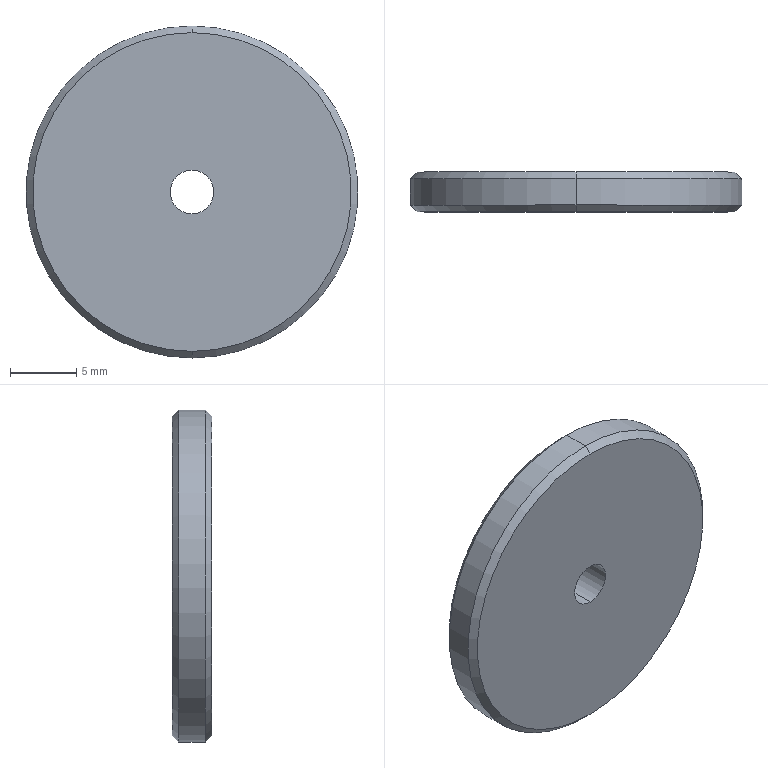Part | STEP file | ND25021-01-JDKM-13-BJ | 1 solid | 10 faces | box 25 x 3 x 25 mm | volume 1428 mm3 | cylinder 4 | cone 4 | plane 2 | commonest cylinder face diameters 3.3 x2 25 x2
STEP:
#1=CARTESIAN_POINT('',(0.,0.,0.));
#2=DIRECTION('',(0.,0.,1.));
#3=DIRECTION('',(1.,0.,0.));
#4=AXIS2_PLACEMENT_3D('',#1,#2,#3);
#5=CARTESIAN_POINT('',(0.,0.,1.65));
#6=VERTEX_POINT('',#5);
#7=CARTESIAN_POINT('',(0.,3.,1.65));
#8=VERTEX_POINT('',#7);
#9=CARTESIAN_POINT('',(0.,3.,1.65));
#10=DIRECTION('',(0.,1.,0.));
#11=VECTOR('',#10,1.);
#12=LINE('',#9,#11);
#13=CARTESIAN_POINT('',(0.,3.,0.));
#14=DIRECTION('',(0.,1.,0.));
#15=DIRECTION('',(0.,0.,1.));
#16=AXIS2_PLACEMENT_3D('',#13,#14,#15);
#17=CYLINDRICAL_SURFACE('',#16,1.65);
#18=CARTESIAN_POINT('',(6.283,0.));
#19=DIRECTION('',(0.,1.));
#20=VECTOR('',#19,1.);
#21=LINE('',#18,#20);
#22=(GEOMETRIC_REPRESENTATION_CONTEXT(2)PARAMETRIC_REPRESENTATION_CONTEXT()REPRESENTATION_CONTEXT('',''));
#23=DEFINITIONAL_REPRESENTATION('',(#21),#22);
#24=PCURVE('',#17,#23);
#25=CARTESIAN_POINT('',(0.,3.,0.));
#26=DIRECTION('',(0.,1.,0.));
#27=DIRECTION('',(0.,0.,1.));
#28=AXIS2_PLACEMENT_3D('',#25,#26,#27);
#29=CYLINDRICAL_SURFACE('',#28,1.65);
#30=CARTESIAN_POINT('',(0.,0.));
#31=DIRECTION('',(0.,1.));
#32=VECTOR('',#31,1.);
#33=LINE('',#30,#32);
#34=(GEOMETRIC_REPRESENTATION_CONTEXT(2)PARAMETRIC_REPRESENTATION_CONTEXT()REPRESENTATION_CONTEXT('',''));
#35=DEFINITIONAL_REPRESENTATION('',(#33),#34);
#36=PCURVE('',#29,#35);
#37=SURFACE_CURVE('',#12,(#24,#36),.PCURVE_S1.);
#38=EDGE_CURVE('',#6,#8,#37,.T.);
#39=ORIENTED_EDGE('',*,*,#38,.T.);
#40=CARTESIAN_POINT('',(0.,3.,-1.65));
#41=VERTEX_POINT('',#40);
#42=CARTESIAN_POINT('',(0.,3.,0.));
#43=DIRECTION('',(0.,1.,0.));
#44=DIRECTION('',(0.,0.,1.));
#45=AXIS2_PLACEMENT_3D('',#42,#43,#44);
#46=CIRCLE('',#45,1.65);
#47=CARTESIAN_POINT('',(0.,0.));
#48=DIRECTION('',(1.,0.));
#49=VECTOR('',#48,1.);
#50=LINE('',#47,#49);
#51=(GEOMETRIC_REPRESENTATION_CONTEXT(2)PARAMETRIC_REPRESENTATION_CONTEXT()REPRESENTATION_CONTEXT('',''));
#52=DEFINITIONAL_REPRESENTATION('',(#50),#51);
#53=PCURVE('',#17,#52);
#54=CARTESIAN_POINT('',(0.,3.,0.));
#55=DIRECTION('',(0.,1.,0.));
#56=DIRECTION('',(0.,0.,1.));
#57=AXIS2_PLACEMENT_3D('',#54,#55,#56);
#58=PLANE('',#57);
#59=CARTESIAN_POINT('',(0.,0.));
#60=DIRECTION('',(1.,0.));
#61=AXIS2_PLACEMENT_2D('',#59,#60);
#62=CIRCLE('',#61,1.65);
#63=(GEOMETRIC_REPRESENTATION_CONTEXT(2)PARAMETRIC_REPRESENTATION_CONTEXT()REPRESENTATION_CONTEXT('',''));
#64=DEFINITIONAL_REPRESENTATION('',(#62),#63);
#65=PCURVE('',#58,#64);
#66=SURFACE_CURVE('',#46,(#53,#65),.PCURVE_S1.);
#67=EDGE_CURVE('',#41,#8,#66,.T.);
#68=ORIENTED_EDGE('',*,*,#67,.F.);
#69=CARTESIAN_POINT('',(0.,0.,-1.65));
#70=VERTEX_POINT('',#69);
#71=CARTESIAN_POINT('',(0.,3.,-1.65));
#72=DIRECTION('',(0.,1.,0.));
#73=VECTOR('',#72,1.);
#74=LINE('',#71,#73);
#75=CARTESIAN_POINT('',(3.142,0.));
#76=DIRECTION('',(0.,1.));
#77=VECTOR('',#76,1.);
#78=LINE('',#75,#77);
#79=(GEOMETRIC_REPRESENTATION_CONTEXT(2)PARAMETRIC_REPRESENTATION_CONTEXT()REPRESENTATION_CONTEXT('',''));
#80=DEFINITIONAL_REPRESENTATION('',(#78),#79);
#81=PCURVE('',#17,#80);
#82=CARTESIAN_POINT('',(3.142,0.));
#83=DIRECTION('',(0.,1.));
#84=VECTOR('',#83,1.);
#85=LINE('',#82,#84);
#86=(GEOMETRIC_REPRESENTATION_CONTEXT(2)PARAMETRIC_REPRESENTATION_CONTEXT()REPRESENTATION_CONTEXT('',''));
#87=DEFINITIONAL_REPRESENTATION('',(#85),#86);
#88=PCURVE('',#29,#87);
#89=SURFACE_CURVE('',#74,(#81,#88),.PCURVE_S1.);
#90=EDGE_CURVE('',#70,#41,#89,.T.);
#91=ORIENTED_EDGE('',*,*,#90,.F.);
#92=CARTESIAN_POINT('',(0.,0.,0.));
#93=DIRECTION('',(0.,1.,0.));
#94=DIRECTION('',(0.,0.,1.));
#95=AXIS2_PLACEMENT_3D('',#92,#93,#94);
#96=CIRCLE('',#95,1.65);
#97=CARTESIAN_POINT('',(0.,-3.));
#98=DIRECTION('',(1.,0.));
#99=VECTOR('',#98,1.);
#100=LINE('',#97,#99);
#101=(GEOMETRIC_REPRESENTATION_CONTEXT(2)PARAMETRIC_REPRESENTATION_CONTEXT()REPRESENTATION_CONTEXT('',''));
#102=DEFINITIONAL_REPRESENTATION('',(#100),#101);
#103=PCURVE('',#17,#102);
#104=CARTESIAN_POINT('',(0.,0.,0.));
#105=DIRECTION('',(0.,1.,0.));
#106=DIRECTION('',(0.,0.,1.));
#107=AXIS2_PLACEMENT_3D('',#104,#105,#106);
#108=PLANE('',#107);
#109=CARTESIAN_POINT('',(0.,0.));
#110=DIRECTION('',(1.,0.));
#111=AXIS2_PLACEMENT_2D('',#109,#110);
#112=CIRCLE('',#111,1.65);
#113=(GEOMETRIC_REPRESENTATION_CONTEXT(2)PARAMETRIC_REPRESENTATION_CONTEXT()REPRESENTATION_CONTEXT('',''));
#114=DEFINITIONAL_REPRESENTATION('',(#112),#113);
#115=PCURVE('',#108,#114);
#116=SURFACE_CURVE('',#96,(#103,#115),.PCURVE_S1.);
#117=EDGE_CURVE('',#70,#6,#116,.T.);
#118=ORIENTED_EDGE('',*,*,#117,.T.);
#119=EDGE_LOOP('',(#39,#68,#91,#118));
#120=FACE_BOUND('',#119,.F.);
#121=ADVANCED_FACE('',(#120),#17,.F.);
#122=CARTESIAN_POINT('',(0.,3.,12.));
#123=VERTEX_POINT('',#122);
#124=CARTESIAN_POINT('',(0.,3.,-12.));
#125=VERTEX_POINT('',#124);
#126=CARTESIAN_POINT('',(0.,3.,0.));
#127=DIRECTION('',(0.,1.,0.));
#128=DIRECTION('',(0.,0.,1.));
#129=AXIS2_PLACEMENT_3D('',#126,#127,#128);
#130=CIRCLE('',#129,12.);
#131=CARTESIAN_POINT('',(0.,3.,0.));
#132=DIRECTION('',(0.,-1.,0.));
#133=DIRECTION('',(0.,0.,-1.));
#134=AXIS2_PLACEMENT_3D('',#131,#132,#133);
#135=CONICAL_SURFACE('',#134,12.,0.7854);
#136=CARTESIAN_POINT('',(3.142,0.));
#137=DIRECTION('',(-1.,0.));
#138=VECTOR('',#137,1.);
#139=LINE('',#136,#138);
#140=(GEOMETRIC_REPRESENTATION_CONTEXT(2)PARAMETRIC_REPRESENTATION_CONTEXT()REPRESENTATION_CONTEXT('',''));
#141=DEFINITIONAL_REPRESENTATION('',(#139),#140);
#142=PCURVE('',#135,#141);
#143=CARTESIAN_POINT('',(0.,0.));
#144=DIRECTION('',(1.,0.));
#145=AXIS2_PLACEMENT_2D('',#143,#144);
#146=CIRCLE('',#145,12.);
#147=(GEOMETRIC_REPRESENTATION_CONTEXT(2)PARAMETRIC_REPRESENTATION_CONTEXT()REPRESENTATION_CONTEXT('',''));
#148=DEFINITIONAL_REPRESENTATION('',(#146),#147);
#149=PCURVE('',#58,#148);
#150=SURFACE_CURVE('',#130,(#142,#149),.PCURVE_S1.);
#151=EDGE_CURVE('',#123,#125,#150,.T.);
#152=ORIENTED_EDGE('',*,*,#151,.F.);
#153=CARTESIAN_POINT('',(0.,2.5,12.5));
#154=VERTEX_POINT('',#153);
#155=CARTESIAN_POINT('',(0.,3.,12.));
#156=DIRECTION('',(0.,-0.7071,0.7071));
#157=VECTOR('',#156,1.);
#158=LINE('',#155,#157);
#159=CARTESIAN_POINT('',(3.142,0.));
#160=DIRECTION('',(0.,1.));
#161=VECTOR('',#160,1.);
#162=LINE('',#159,#161);
#163=(GEOMETRIC_REPRESENTATION_CONTEXT(2)PARAMETRIC_REPRESENTATION_CONTEXT()REPRESENTATION_CONTEXT('',''));
#164=DEFINITIONAL_REPRESENTATION('',(#162),#163);
#165=PCURVE('',#135,#164);
#166=CARTESIAN_POINT('',(0.,3.,0.));
#167=DIRECTION('',(0.,-1.,0.));
#168=DIRECTION('',(0.,0.,-1.));
#169=AXIS2_PLACEMENT_3D('',#166,#167,#168);
#170=CONICAL_SURFACE('',#169,12.,0.7854);
#171=CARTESIAN_POINT('',(3.142,0.));
#172=DIRECTION('',(0.,1.));
#173=VECTOR('',#172,1.);
#174=LINE('',#171,#173);
#175=(GEOMETRIC_REPRESENTATION_CONTEXT(2)PARAMETRIC_REPRESENTATION_CONTEXT()REPRESENTATION_CONTEXT('',''));
#176=DEFINITIONAL_REPRESENTATION('',(#174),#175);
#177=PCURVE('',#170,#176);
#178=SURFACE_CURVE('',#158,(#165,#177),.PCURVE_S1.);
#179=EDGE_CURVE('',#123,#154,#178,.T.);
#180=ORIENTED_EDGE('',*,*,#179,.T.);
#181=CARTESIAN_POINT('',(0.,2.5,-12.5));
#182=VERTEX_POINT('',#181);
#183=CARTESIAN_POINT('',(0.,2.5,0.));
#184=DIRECTION('',(0.,-1.,0.));
#185=DIRECTION('',(0.,0.,1.));
#186=AXIS2_PLACEMENT_3D('',#183,#184,#185);
#187=CIRCLE('',#186,12.5);
#188=CARTESIAN_POINT('',(-3.142,0.5));
#189=DIRECTION('',(1.,0.));
#190=VECTOR('',#189,1.);
#191=LINE('',#188,#190);
#192=(GEOMETRIC_REPRESENTATION_CONTEXT(2)PARAMETRIC_REPRESENTATION_CONTEXT()REPRESENTATION_CONTEXT('',''));
#193=DEFINITIONAL_REPRESENTATION('',(#191),#192);
#194=PCURVE('',#135,#193);
#195=CARTESIAN_POINT('',(0.,3.,0.));
#196=DIRECTION('',(0.,-1.,0.));
#197=DIRECTION('',(0.,0.,-1.));
#198=AXIS2_PLACEMENT_3D('',#195,#196,#197);
#199=CYLINDRICAL_SURFACE('',#198,12.5);
#200=CARTESIAN_POINT('',(-3.142,0.5));
#201=DIRECTION('',(1.,0.));
#202=VECTOR('',#201,1.);
#203=LINE('',#200,#202);
#204=(GEOMETRIC_REPRESENTATION_CONTEXT(2)PARAMETRIC_REPRESENTATION_CONTEXT()REPRESENTATION_CONTEXT('',''));
#205=DEFINITIONAL_REPRESENTATION('',(#203),#204);
#206=PCURVE('',#199,#205);
#207=SURFACE_CURVE('',#187,(#194,#206),.PCURVE_S1.);
#208=EDGE_CURVE('',#182,#154,#207,.T.);
#209=ORIENTED_EDGE('',*,*,#208,.F.);
#210=CARTESIAN_POINT('',(0.,3.,-12.));
#211=DIRECTION('',(0.,-0.7071,-0.7071));
#212=VECTOR('',#211,1.);
#213=LINE('',#210,#212);
#214=CARTESIAN_POINT('',(0.,0.));
#215=DIRECTION('',(0.,1.));
#216=VECTOR('',#215,1.);
#217=LINE('',#214,#216);
#218=(GEOMETRIC_REPRESENTATION_CONTEXT(2)PARAMETRIC_REPRESENTATION_CONTEXT()REPRESENTATION_CONTEXT('',''));
#219=DEFINITIONAL_REPRESENTATION('',(#217),#218);
#220=PCURVE('',#135,#219);
#221=CARTESIAN_POINT('',(6.283,0.));
#222=DIRECTION('',(0.,1.));
#223=VECTOR('',#222,1.);
#224=LINE('',#221,#223);
#225=(GEOMETRIC_REPRESENTATION_CONTEXT(2)PARAMETRIC_REPRESENTATION_CONTEXT()REPRESENTATION_CONTEXT('',''));
#226=DEFINITIONAL_REPRESENTATION('',(#224),#225);
#227=PCURVE('',#170,#226);
#228=SURFACE_CURVE('',#213,(#220,#227),.PCURVE_S1.);
#229=EDGE_CURVE('',#125,#182,#228,.T.);
#230=ORIENTED_EDGE('',*,*,#229,.F.);
#231=EDGE_LOOP('',(#152,#180,#209,#230));
#232=FACE_BOUND('',#231,.T.);
#233=ADVANCED_FACE('',(#232),#135,.T.);
#234=CARTESIAN_POINT('',(0.,0.,-12.));
#235=VERTEX_POINT('',#234);
#236=CARTESIAN_POINT('',(0.,0.,12.));
#237=VERTEX_POINT('',#236);
#238=CARTESIAN_POINT('',(0.,0.,0.));
#239=DIRECTION('',(0.,-1.,0.));
#240=DIRECTION('',(0.,0.,1.));
#241=AXIS2_PLACEMENT_3D('',#238,#239,#240);
#242=CIRCLE('',#241,12.);
#243=CARTESIAN_POINT('',(0.,0.5,0.));
#244=DIRECTION('',(0.,1.,0.));
#245=DIRECTION('',(0.,0.,1.));
#246=AXIS2_PLACEMENT_3D('',#243,#244,#245);
#247=CONICAL_SURFACE('',#246,12.5,0.7854);
#248=CARTESIAN_POINT('',(6.283,-0.5));
#249=DIRECTION('',(-1.,0.));
#250=VECTOR('',#249,1.);
#251=LINE('',#248,#250);
#252=(GEOMETRIC_REPRESENTATION_CONTEXT(2)PARAMETRIC_REPRESENTATION_CONTEXT()REPRESENTATION_CONTEXT('',''));
#253=DEFINITIONAL_REPRESENTATION('',(#251),#252);
#254=PCURVE('',#247,#253);
#255=CARTESIAN_POINT('',(12.,0.));
#256=CARTESIAN_POINT('',(12.,-20.785));
#257=CARTESIAN_POINT('',(-6.,-10.392));
#258=CARTESIAN_POINT('',(-24.,0.));
#259=CARTESIAN_POINT('',(-6.,10.392));
#260=CARTESIAN_POINT('',(12.,20.785));
#261=CARTESIAN_POINT('',(12.,0.));
#262=(BOUNDED_CURVE()B_SPLINE_CURVE(2,(#255,#256,#257,#258,#259,#260,#261),.UNSPECIFIED.,.T.,.F.)B_SPLINE_CURVE_WITH_KNOTS((1,2,2,2,2,1),(-2.094,0.,2.094,4.189,6.283,8.378),.UNSPECIFIED.)CURVE()GEOMETRIC_REPRESENTATION_ITEM()RATIONAL_B_SPLINE_CURVE((1.,0.5,1.,0.5,1.,0.5,1.))REPRESENTATION_ITEM(''));
#263=(GEOMETRIC_REPRESENTATION_CONTEXT(2)PARAMETRIC_REPRESENTATION_CONTEXT()REPRESENTATION_CONTEXT('',''));
#264=DEFINITIONAL_REPRESENTATION('',(#262),#263);
#265=PCURVE('',#108,#264);
#266=SURFACE_CURVE('',#242,(#254,#265),.PCURVE_S1.);
#267=EDGE_CURVE('',#235,#237,#266,.T.);
#268=ORIENTED_EDGE('',*,*,#267,.F.);
#269=CARTESIAN_POINT('',(0.,0.5,-12.5));
#270=VERTEX_POINT('',#269);
#271=CARTESIAN_POINT('',(0.,0.5,-12.5));
#272=DIRECTION('',(0.,0.7071,-0.7071));
#273=VECTOR('',#272,1.);
#274=LINE('',#271,#273);
#275=CARTESIAN_POINT('',(3.142,0.));
#276=DIRECTION('',(0.,1.));
#277=VECTOR('',#276,1.);
#278=LINE('',#275,#277);
#279=(GEOMETRIC_REPRESENTATION_CONTEXT(2)PARAMETRIC_REPRESENTATION_CONTEXT()REPRESENTATION_CONTEXT('',''));
#280=DEFINITIONAL_REPRESENTATION('',(#278),#279);
#281=PCURVE('',#247,#280);
#282=CARTESIAN_POINT('',(0.,0.5,0.));
#283=DIRECTION('',(0.,1.,0.));
#284=DIRECTION('',(0.,0.,1.));
#285=AXIS2_PLACEMENT_3D('',#282,#283,#284);
#286=CONICAL_SURFACE('',#285,12.5,0.7854);
#287=CARTESIAN_POINT('',(3.142,0.));
#288=DIRECTION('',(0.,1.));
#289=VECTOR('',#288,1.);
#290=LINE('',#287,#289);
#291=(GEOMETRIC_REPRESENTATION_CONTEXT(2)PARAMETRIC_REPRESENTATION_CONTEXT()REPRESENTATION_CONTEXT('',''));
#292=DEFINITIONAL_REPRESENTATION('',(#290),#291);
#293=PCURVE('',#286,#292);
#294=SURFACE_CURVE('',#274,(#281,#293),.PCURVE_S1.);
#295=EDGE_CURVE('',#235,#270,#294,.T.);
#296=ORIENTED_EDGE('',*,*,#295,.T.);
#297=CARTESIAN_POINT('',(0.,0.5,12.5));
#298=VERTEX_POINT('',#297);
#299=CARTESIAN_POINT('',(0.,0.5,0.));
#300=DIRECTION('',(0.,1.,0.));
#301=DIRECTION('',(0.,0.,1.));
#302=AXIS2_PLACEMENT_3D('',#299,#300,#301);
#303=CIRCLE('',#302,12.5);
#304=CARTESIAN_POINT('',(0.,0.));
#305=DIRECTION('',(1.,0.));
#306=VECTOR('',#305,1.);
#307=LINE('',#304,#306);
#308=(GEOMETRIC_REPRESENTATION_CONTEXT(2)PARAMETRIC_REPRESENTATION_CONTEXT()REPRESENTATION_CONTEXT('',''));
#309=DEFINITIONAL_REPRESENTATION('',(#307),#308);
#310=PCURVE('',#247,#309);
#311=CARTESIAN_POINT('',(3.142,2.5));
#312=DIRECTION('',(-1.,0.));
#313=VECTOR('',#312,1.);
#314=LINE('',#311,#313);
#315=(GEOMETRIC_REPRESENTATION_CONTEXT(2)PARAMETRIC_REPRESENTATION_CONTEXT()REPRESENTATION_CONTEXT('',''));
#316=DEFINITIONAL_REPRESENTATION('',(#314),#315);
#317=PCURVE('',#199,#316);
#318=SURFACE_CURVE('',#303,(#310,#317),.PCURVE_S1.);
#319=EDGE_CURVE('',#298,#270,#318,.T.);
#320=ORIENTED_EDGE('',*,*,#319,.F.);
#321=CARTESIAN_POINT('',(0.,0.5,12.5));
#322=DIRECTION('',(0.,0.7071,0.7071));
#323=VECTOR('',#322,1.);
#324=LINE('',#321,#323);
#325=CARTESIAN_POINT('',(0.,0.));
#326=DIRECTION('',(0.,1.));
#327=VECTOR('',#326,1.);
#328=LINE('',#325,#327);
#329=(GEOMETRIC_REPRESENTATION_CONTEXT(2)PARAMETRIC_REPRESENTATION_CONTEXT()REPRESENTATION_CONTEXT('',''));
#330=DEFINITIONAL_REPRESENTATION('',(#328),#329);
#331=PCURVE('',#247,#330);
#332=CARTESIAN_POINT('',(6.283,0.));
#333=DIRECTION('',(0.,1.));
#334=VECTOR('',#333,1.);
#335=LINE('',#332,#334);
#336=(GEOMETRIC_REPRESENTATION_CONTEXT(2)PARAMETRIC_REPRESENTATION_CONTEXT()REPRESENTATION_CONTEXT('',''));
#337=DEFINITIONAL_REPRESENTATION('',(#335),#336);
#338=PCURVE('',#286,#337);
#339=SURFACE_CURVE('',#324,(#331,#338),.PCURVE_S1.);
#340=EDGE_CURVE('',#237,#298,#339,.T.);
#341=ORIENTED_EDGE('',*,*,#340,.F.);
#342=EDGE_LOOP('',(#268,#296,#320,#341));
#343=FACE_BOUND('',#342,.T.);
#344=ADVANCED_FACE('',(#343),#247,.T.);
#345=ORIENTED_EDGE('',*,*,#208,.T.);
#346=CARTESIAN_POINT('',(0.,3.,12.5));
#347=DIRECTION('',(0.,-1.,0.));
#348=VECTOR('',#347,1.);
#349=LINE('',#346,#348);
#350=CARTESIAN_POINT('',(3.142,0.));
#351=DIRECTION('',(0.,1.));
#352=VECTOR('',#351,1.);
#353=LINE('',#350,#352);
#354=(GEOMETRIC_REPRESENTATION_CONTEXT(2)PARAMETRIC_REPRESENTATION_CONTEXT()REPRESENTATION_CONTEXT('',''));
#355=DEFINITIONAL_REPRESENTATION('',(#353),#354);
#356=PCURVE('',#199,#355);
#357=CARTESIAN_POINT('',(0.,3.,0.));
#358=DIRECTION('',(0.,-1.,0.));
#359=DIRECTION('',(0.,0.,-1.));
#360=AXIS2_PLACEMENT_3D('',#357,#358,#359);
#361=CYLINDRICAL_SURFACE('',#360,12.5);
#362=CARTESIAN_POINT('',(3.142,0.));
#363=DIRECTION('',(0.,1.));
#364=VECTOR('',#363,1.);
#365=LINE('',#362,#364);
#366=(GEOMETRIC_REPRESENTATION_CONTEXT(2)PARAMETRIC_REPRESENTATION_CONTEXT()REPRESENTATION_CONTEXT('',''));
#367=DEFINITIONAL_REPRESENTATION('',(#365),#366);
#368=PCURVE('',#361,#367);
#369=SURFACE_CURVE('',#349,(#356,#368),.PCURVE_S1.);
#370=EDGE_CURVE('',#154,#298,#369,.T.);
#371=ORIENTED_EDGE('',*,*,#370,.T.);
#372=ORIENTED_EDGE('',*,*,#319,.T.);
#373=CARTESIAN_POINT('',(0.,3.,-12.5));
#374=DIRECTION('',(0.,-1.,0.));
#375=VECTOR('',#374,1.);
#376=LINE('',#373,#375);
#377=CARTESIAN_POINT('',(0.,0.));
#378=DIRECTION('',(0.,1.));
#379=VECTOR('',#378,1.);
#380=LINE('',#377,#379);
#381=(GEOMETRIC_REPRESENTATION_CONTEXT(2)PARAMETRIC_REPRESENTATION_CONTEXT()REPRESENTATION_CONTEXT('',''));
#382=DEFINITIONAL_REPRESENTATION('',(#380),#381);
#383=PCURVE('',#199,#382);
#384=CARTESIAN_POINT('',(6.283,0.));
#385=DIRECTION('',(0.,1.));
#386=VECTOR('',#385,1.);
#387=LINE('',#384,#386);
#388=(GEOMETRIC_REPRESENTATION_CONTEXT(2)PARAMETRIC_REPRESENTATION_CONTEXT()REPRESENTATION_CONTEXT('',''));
#389=DEFINITIONAL_REPRESENTATION('',(#387),#388);
#390=PCURVE('',#361,#389);
#391=SURFACE_CURVE('',#376,(#383,#390),.PCURVE_S1.);
#392=EDGE_CURVE('',#182,#270,#391,.T.);
#393=ORIENTED_EDGE('',*,*,#392,.F.);
#394=EDGE_LOOP('',(#345,#371,#372,#393));
#395=FACE_BOUND('',#394,.T.);
#396=ADVANCED_FACE('',(#395),#199,.T.);
#397=ORIENTED_EDGE('',*,*,#370,.F.);
#398=CARTESIAN_POINT('',(0.,2.5,0.));
#399=DIRECTION('',(0.,-1.,0.));
#400=DIRECTION('',(0.,0.,1.));
#401=AXIS2_PLACEMENT_3D('',#398,#399,#400);
#402=CIRCLE('',#401,12.5);
#403=CARTESIAN_POINT('',(3.142,0.5));
#404=DIRECTION('',(1.,0.));
#405=VECTOR('',#404,1.);
#406=LINE('',#403,#405);
#407=(GEOMETRIC_REPRESENTATION_CONTEXT(2)PARAMETRIC_REPRESENTATION_CONTEXT()REPRESENTATION_CONTEXT('',''));
#408=DEFINITIONAL_REPRESENTATION('',(#406),#407);
#409=PCURVE('',#361,#408);
#410=CARTESIAN_POINT('',(3.142,0.5));
#411=DIRECTION('',(1.,0.));
#412=VECTOR('',#411,1.);
#413=LINE('',#410,#412);
#414=(GEOMETRIC_REPRESENTATION_CONTEXT(2)PARAMETRIC_REPRESENTATION_CONTEXT()REPRESENTATION_CONTEXT('',''));
#415=DEFINITIONAL_REPRESENTATION('',(#413),#414);
#416=PCURVE('',#170,#415);
#417=SURFACE_CURVE('',#402,(#409,#416),.PCURVE_S1.);
#418=EDGE_CURVE('',#154,#182,#417,.T.);
#419=ORIENTED_EDGE('',*,*,#418,.T.);
#420=ORIENTED_EDGE('',*,*,#392,.T.);
#421=CARTESIAN_POINT('',(0.,0.5,0.));
#422=DIRECTION('',(0.,1.,0.));
#423=DIRECTION('',(0.,0.,1.));
#424=AXIS2_PLACEMENT_3D('',#421,#422,#423);
#425=CIRCLE('',#424,12.5);
#426=CARTESIAN_POINT('',(9.425,2.5));
#427=DIRECTION('',(-1.,0.));
#428=VECTOR('',#427,1.);
#429=LINE('',#426,#428);
#430=(GEOMETRIC_REPRESENTATION_CONTEXT(2)PARAMETRIC_REPRESENTATION_CONTEXT()REPRESENTATION_CONTEXT('',''));
#431=DEFINITIONAL_REPRESENTATION('',(#429),#430);
#432=PCURVE('',#361,#431);
#433=CARTESIAN_POINT('',(0.,0.));
#434=DIRECTION('',(1.,0.));
#435=VECTOR('',#434,1.);
#436=LINE('',#433,#435);
#437=(GEOMETRIC_REPRESENTATION_CONTEXT(2)PARAMETRIC_REPRESENTATION_CONTEXT()REPRESENTATION_CONTEXT('',''));
#438=DEFINITIONAL_REPRESENTATION('',(#436),#437);
#439=PCURVE('',#286,#438);
#440=SURFACE_CURVE('',#425,(#432,#439),.PCURVE_S1.);
#441=EDGE_CURVE('',#270,#298,#440,.T.);
#442=ORIENTED_EDGE('',*,*,#441,.T.);
#443=EDGE_LOOP('',(#397,#419,#420,#442));
#444=FACE_BOUND('',#443,.T.);
#445=ADVANCED_FACE('',(#444),#361,.T.);
#446=CARTESIAN_POINT('',(0.,3.,0.));
#447=DIRECTION('',(0.,1.,0.));
#448=DIRECTION('',(0.,0.,1.));
#449=AXIS2_PLACEMENT_3D('',#446,#447,#448);
#450=CIRCLE('',#449,1.65);
#451=CARTESIAN_POINT('',(0.,0.));
#452=DIRECTION('',(1.,0.));
#453=AXIS2_PLACEMENT_2D('',#451,#452);
#454=CIRCLE('',#453,1.65);
#455=(GEOMETRIC_REPRESENTATION_CONTEXT(2)PARAMETRIC_REPRESENTATION_CONTEXT()REPRESENTATION_CONTEXT('',''));
#456=DEFINITIONAL_REPRESENTATION('',(#454),#455);
#457=PCURVE('',#58,#456);
#458=CARTESIAN_POINT('',(0.,0.));
#459=DIRECTION('',(1.,0.));
#460=VECTOR('',#459,1.);
#461=LINE('',#458,#460);
#462=(GEOMETRIC_REPRESENTATION_CONTEXT(2)PARAMETRIC_REPRESENTATION_CONTEXT()REPRESENTATION_CONTEXT('',''));
#463=DEFINITIONAL_REPRESENTATION('',(#461),#462);
#464=PCURVE('',#29,#463);
#465=SURFACE_CURVE('',#450,(#457,#464),.PCURVE_S1.);
#466=EDGE_CURVE('',#8,#41,#465,.T.);
#467=ORIENTED_EDGE('',*,*,#466,.F.);
#468=ORIENTED_EDGE('',*,*,#67,.F.);
#469=EDGE_LOOP('',(#467,#468));
#470=FACE_BOUND('',#469,.T.);
#471=CARTESIAN_POINT('',(0.,3.,0.));
#472=DIRECTION('',(0.,1.,0.));
#473=DIRECTION('',(0.,0.,1.));
#474=AXIS2_PLACEMENT_3D('',#471,#472,#473);
#475=CIRCLE('',#474,12.);
#476=CARTESIAN_POINT('',(0.,0.));
#477=DIRECTION('',(1.,0.));
#478=AXIS2_PLACEMENT_2D('',#476,#477);
#479=CIRCLE('',#478,12.);
#480=(GEOMETRIC_REPRESENTATION_CONTEXT(2)PARAMETRIC_REPRESENTATION_CONTEXT()REPRESENTATION_CONTEXT('',''));
#481=DEFINITIONAL_REPRESENTATION('',(#479),#480);
#482=PCURVE('',#58,#481);
#483=CARTESIAN_POINT('',(9.425,0.));
#484=DIRECTION('',(-1.,0.));
#485=VECTOR('',#484,1.);
#486=LINE('',#483,#485);
#487=(GEOMETRIC_REPRESENTATION_CONTEXT(2)PARAMETRIC_REPRESENTATION_CONTEXT()REPRESENTATION_CONTEXT('',''));
#488=DEFINITIONAL_REPRESENTATION('',(#486),#487);
#489=PCURVE('',#170,#488);
#490=SURFACE_CURVE('',#475,(#482,#489),.PCURVE_S1.);
#491=EDGE_CURVE('',#125,#123,#490,.T.);
#492=ORIENTED_EDGE('',*,*,#491,.T.);
#493=ORIENTED_EDGE('',*,*,#151,.T.);
#494=EDGE_LOOP('',(#492,#493));
#495=FACE_BOUND('',#494,.T.);
#496=ADVANCED_FACE('',(#470,#495),#58,.T.);
#497=CARTESIAN_POINT('',(0.,0.,0.));
#498=DIRECTION('',(0.,1.,0.));
#499=DIRECTION('',(0.,0.,1.));
#500=AXIS2_PLACEMENT_3D('',#497,#498,#499);
#501=CIRCLE('',#500,1.65);
#502=CARTESIAN_POINT('',(0.,0.));
#503=DIRECTION('',(1.,0.));
#504=AXIS2_PLACEMENT_2D('',#502,#503);
#505=CIRCLE('',#504,1.65);
#506=(GEOMETRIC_REPRESENTATION_CONTEXT(2)PARAMETRIC_REPRESENTATION_CONTEXT()REPRESENTATION_CONTEXT('',''));
#507=DEFINITIONAL_REPRESENTATION('',(#505),#506);
#508=PCURVE('',#108,#507);
#509=CARTESIAN_POINT('',(0.,-3.));
#510=DIRECTION('',(1.,0.));
#511=VECTOR('',#510,1.);
#512=LINE('',#509,#511);
#513=(GEOMETRIC_REPRESENTATION_CONTEXT(2)PARAMETRIC_REPRESENTATION_CONTEXT()REPRESENTATION_CONTEXT('',''));
#514=DEFINITIONAL_REPRESENTATION('',(#512),#513);
#515=PCURVE('',#29,#514);
#516=SURFACE_CURVE('',#501,(#508,#515),.PCURVE_S1.);
#517=EDGE_CURVE('',#6,#70,#516,.T.);
#518=ORIENTED_EDGE('',*,*,#517,.T.);
#519=ORIENTED_EDGE('',*,*,#117,.T.);
#520=EDGE_LOOP('',(#518,#519));
#521=FACE_BOUND('',#520,.T.);
#522=CARTESIAN_POINT('',(0.,0.,0.));
#523=DIRECTION('',(0.,-1.,0.));
#524=DIRECTION('',(0.,0.,1.));
#525=AXIS2_PLACEMENT_3D('',#522,#523,#524);
#526=CIRCLE('',#525,12.);
#527=CARTESIAN_POINT('',(12.,0.));
#528=CARTESIAN_POINT('',(12.,-20.785));
#529=CARTESIAN_POINT('',(-6.,-10.392));
#530=CARTESIAN_POINT('',(-24.,0.));
#531=CARTESIAN_POINT('',(-6.,10.392));
#532=CARTESIAN_POINT('',(12.,20.785));
#533=CARTESIAN_POINT('',(12.,0.));
#534=(BOUNDED_CURVE()B_SPLINE_CURVE(2,(#527,#528,#529,#530,#531,#532,#533),.UNSPECIFIED.,.T.,.F.)B_SPLINE_CURVE_WITH_KNOTS((1,2,2,2,2,1),(-2.094,0.,2.094,4.189,6.283,8.378),.UNSPECIFIED.)CURVE()GEOMETRIC_REPRESENTATION_ITEM()RATIONAL_B_SPLINE_CURVE((1.,0.5,1.,0.5,1.,0.5,1.))REPRESENTATION_ITEM(''));
#535=(GEOMETRIC_REPRESENTATION_CONTEXT(2)PARAMETRIC_REPRESENTATION_CONTEXT()REPRESENTATION_CONTEXT('',''));
#536=DEFINITIONAL_REPRESENTATION('',(#534),#535);
#537=PCURVE('',#108,#536);
#538=CARTESIAN_POINT('',(6.283,-0.5));
#539=DIRECTION('',(-1.,0.));
#540=VECTOR('',#539,1.);
#541=LINE('',#538,#540);
#542=(GEOMETRIC_REPRESENTATION_CONTEXT(2)PARAMETRIC_REPRESENTATION_CONTEXT()REPRESENTATION_CONTEXT('',''));
#543=DEFINITIONAL_REPRESENTATION('',(#541),#542);
#544=PCURVE('',#286,#543);
#545=SURFACE_CURVE('',#526,(#537,#544),.PCURVE_S1.);
#546=EDGE_CURVE('',#237,#235,#545,.T.);
#547=ORIENTED_EDGE('',*,*,#546,.T.);
#548=ORIENTED_EDGE('',*,*,#267,.T.);
#549=EDGE_LOOP('',(#547,#548));
#550=FACE_BOUND('',#549,.T.);
#551=ADVANCED_FACE('',(#521,#550),#108,.F.);
#552=ORIENTED_EDGE('',*,*,#295,.F.);
#553=ORIENTED_EDGE('',*,*,#546,.F.);
#554=ORIENTED_EDGE('',*,*,#340,.T.);
#555=ORIENTED_EDGE('',*,*,#441,.F.);
#556=EDGE_LOOP('',(#552,#553,#554,#555));
#557=FACE_BOUND('',#556,.T.);
#558=ADVANCED_FACE('',(#557),#286,.T.);
#559=ORIENTED_EDGE('',*,*,#179,.F.);
#560=ORIENTED_EDGE('',*,*,#491,.F.);
#561=ORIENTED_EDGE('',*,*,#229,.T.);
#562=ORIENTED_EDGE('',*,*,#418,.F.);
#563=EDGE_LOOP('',(#559,#560,#561,#562));
#564=FACE_BOUND('',#563,.T.);
#565=ADVANCED_FACE('',(#564),#170,.T.);
#566=ORIENTED_EDGE('',*,*,#466,.F.);
#567=ORIENTED_EDGE('',*,*,#38,.F.);
#568=ORIENTED_EDGE('',*,*,#517,.T.);
#569=ORIENTED_EDGE('',*,*,#90,.T.);
#570=EDGE_LOOP('',(#566,#567,#568,#569));
#571=FACE_BOUND('',#570,.F.);
#572=ADVANCED_FACE('',(#571),#29,.F.);
#573=CLOSED_SHELL('',(#121,#233,#344,#396,#445,#496,#551,#558,#565,#572));
#574=MANIFOLD_SOLID_BREP('',#573);
#575=(LENGTH_UNIT()NAMED_UNIT(*)SI_UNIT(.MILLI.,.METRE.));
#576=UNCERTAINTY_MEASURE_WITH_UNIT(LENGTH_MEASURE(0.0000001),#575,'','');
#577=(NAMED_UNIT(*)PLANE_ANGLE_UNIT()SI_UNIT($,.RADIAN.));
#578=(NAMED_UNIT(*)SI_UNIT($,.STERADIAN.)SOLID_ANGLE_UNIT());
#579=(GEOMETRIC_REPRESENTATION_CONTEXT(3)GLOBAL_UNCERTAINTY_ASSIGNED_CONTEXT((#576))GLOBAL_UNIT_ASSIGNED_CONTEXT((#575,#577,#578))REPRESENTATION_CONTEXT('',''));
#580=ADVANCED_BREP_SHAPE_REPRESENTATION('',(#4,#574),#579);